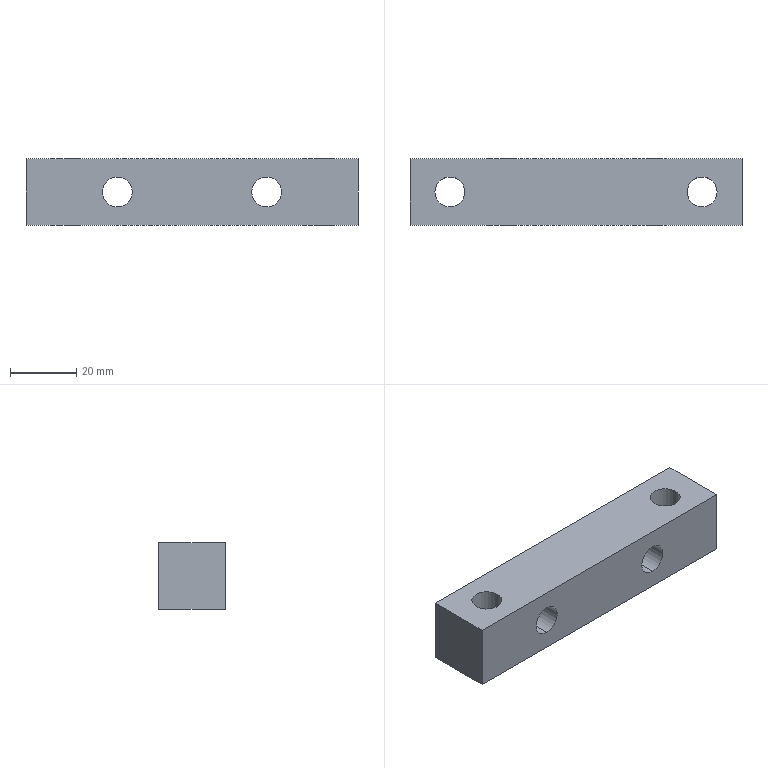Part | STEP file | 0244_218_Block | 1 solid | 14 faces | box 100 x 20 x 20 mm | volume 34911 mm3 | cylinder 8 | plane 6 | commonest cylinder face diameters 9 x8
STEP:
#1=CARTESIAN_POINT('',(0.,0.,0.));
#2=DIRECTION('',(0.,0.,1.));
#3=DIRECTION('',(1.,0.,0.));
#4=AXIS2_PLACEMENT_3D('',#1,#2,#3);
#5=CARTESIAN_POINT('',(-22.5,0.,5.5));
#6=VERTEX_POINT('',#5);
#7=CARTESIAN_POINT('',(-22.5,-20.,5.5));
#8=VERTEX_POINT('',#7);
#9=CARTESIAN_POINT('',(-22.5,-20.,5.5));
#10=DIRECTION('',(0.,-1.,0.));
#11=VECTOR('',#10,1.);
#12=LINE('',#9,#11);
#13=CARTESIAN_POINT('',(-22.5,-20.,10.));
#14=DIRECTION('',(0.,-1.,0.));
#15=DIRECTION('',(0.,0.,-1.));
#16=AXIS2_PLACEMENT_3D('',#13,#14,#15);
#17=CYLINDRICAL_SURFACE('',#16,4.5);
#18=CARTESIAN_POINT('',(6.283,0.));
#19=DIRECTION('',(0.,1.));
#20=VECTOR('',#19,1.);
#21=LINE('',#18,#20);
#22=(GEOMETRIC_REPRESENTATION_CONTEXT(2)PARAMETRIC_REPRESENTATION_CONTEXT()REPRESENTATION_CONTEXT('',''));
#23=DEFINITIONAL_REPRESENTATION('',(#21),#22);
#24=PCURVE('',#17,#23);
#25=CARTESIAN_POINT('',(-22.5,-20.,10.));
#26=DIRECTION('',(0.,-1.,0.));
#27=DIRECTION('',(0.,0.,-1.));
#28=AXIS2_PLACEMENT_3D('',#25,#26,#27);
#29=CYLINDRICAL_SURFACE('',#28,4.5);
#30=CARTESIAN_POINT('',(0.,0.));
#31=DIRECTION('',(0.,1.));
#32=VECTOR('',#31,1.);
#33=LINE('',#30,#32);
#34=(GEOMETRIC_REPRESENTATION_CONTEXT(2)PARAMETRIC_REPRESENTATION_CONTEXT()REPRESENTATION_CONTEXT('',''));
#35=DEFINITIONAL_REPRESENTATION('',(#33),#34);
#36=PCURVE('',#29,#35);
#37=SURFACE_CURVE('',#12,(#24,#36),.PCURVE_S1.);
#38=EDGE_CURVE('',#6,#8,#37,.T.);
#39=ORIENTED_EDGE('',*,*,#38,.T.);
#40=CARTESIAN_POINT('',(-22.5,-20.,14.5));
#41=VERTEX_POINT('',#40);
#42=CARTESIAN_POINT('',(-22.5,-20.,10.));
#43=DIRECTION('',(0.,-1.,0.));
#44=DIRECTION('',(0.,0.,-1.));
#45=AXIS2_PLACEMENT_3D('',#42,#43,#44);
#46=CIRCLE('',#45,4.5);
#47=CARTESIAN_POINT('',(0.,0.));
#48=DIRECTION('',(1.,0.));
#49=VECTOR('',#48,1.);
#50=LINE('',#47,#49);
#51=(GEOMETRIC_REPRESENTATION_CONTEXT(2)PARAMETRIC_REPRESENTATION_CONTEXT()REPRESENTATION_CONTEXT('',''));
#52=DEFINITIONAL_REPRESENTATION('',(#50),#51);
#53=PCURVE('',#17,#52);
#54=CARTESIAN_POINT('',(-50.,-20.,20.));
#55=DIRECTION('',(0.,1.,0.));
#56=DIRECTION('',(-1.,0.,0.));
#57=AXIS2_PLACEMENT_3D('',#54,#55,#56);
#58=PLANE('',#57);
#59=CARTESIAN_POINT('',(-27.5,-14.5));
#60=CARTESIAN_POINT('',(-35.294,-14.5));
#61=CARTESIAN_POINT('',(-31.397,-7.75));
#62=CARTESIAN_POINT('',(-27.5,-1.));
#63=CARTESIAN_POINT('',(-23.603,-7.75));
#64=CARTESIAN_POINT('',(-19.706,-14.5));
#65=CARTESIAN_POINT('',(-27.5,-14.5));
#66=(BOUNDED_CURVE()B_SPLINE_CURVE(2,(#59,#60,#61,#62,#63,#64,#65),.UNSPECIFIED.,.T.,.F.)B_SPLINE_CURVE_WITH_KNOTS((1,2,2,2,2,1),(-2.094,0.,2.094,4.189,6.283,8.378),.UNSPECIFIED.)CURVE()GEOMETRIC_REPRESENTATION_ITEM()RATIONAL_B_SPLINE_CURVE((1.,0.5,1.,0.5,1.,0.5,1.))REPRESENTATION_ITEM(''));
#67=(GEOMETRIC_REPRESENTATION_CONTEXT(2)PARAMETRIC_REPRESENTATION_CONTEXT()REPRESENTATION_CONTEXT('',''));
#68=DEFINITIONAL_REPRESENTATION('',(#66),#67);
#69=PCURVE('',#58,#68);
#70=SURFACE_CURVE('',#46,(#53,#69),.PCURVE_S1.);
#71=EDGE_CURVE('',#41,#8,#70,.T.);
#72=ORIENTED_EDGE('',*,*,#71,.F.);
#73=CARTESIAN_POINT('',(-22.5,0.,14.5));
#74=VERTEX_POINT('',#73);
#75=CARTESIAN_POINT('',(-22.5,-20.,14.5));
#76=DIRECTION('',(0.,-1.,0.));
#77=VECTOR('',#76,1.);
#78=LINE('',#75,#77);
#79=CARTESIAN_POINT('',(3.142,0.));
#80=DIRECTION('',(0.,1.));
#81=VECTOR('',#80,1.);
#82=LINE('',#79,#81);
#83=(GEOMETRIC_REPRESENTATION_CONTEXT(2)PARAMETRIC_REPRESENTATION_CONTEXT()REPRESENTATION_CONTEXT('',''));
#84=DEFINITIONAL_REPRESENTATION('',(#82),#83);
#85=PCURVE('',#17,#84);
#86=CARTESIAN_POINT('',(3.142,0.));
#87=DIRECTION('',(0.,1.));
#88=VECTOR('',#87,1.);
#89=LINE('',#86,#88);
#90=(GEOMETRIC_REPRESENTATION_CONTEXT(2)PARAMETRIC_REPRESENTATION_CONTEXT()REPRESENTATION_CONTEXT('',''));
#91=DEFINITIONAL_REPRESENTATION('',(#89),#90);
#92=PCURVE('',#29,#91);
#93=SURFACE_CURVE('',#78,(#85,#92),.PCURVE_S1.);
#94=EDGE_CURVE('',#74,#41,#93,.T.);
#95=ORIENTED_EDGE('',*,*,#94,.F.);
#96=CARTESIAN_POINT('',(-22.5,0.,10.));
#97=DIRECTION('',(0.,-1.,0.));
#98=DIRECTION('',(0.,0.,-1.));
#99=AXIS2_PLACEMENT_3D('',#96,#97,#98);
#100=CIRCLE('',#99,4.5);
#101=CARTESIAN_POINT('',(0.,-20.));
#102=DIRECTION('',(1.,0.));
#103=VECTOR('',#102,1.);
#104=LINE('',#101,#103);
#105=(GEOMETRIC_REPRESENTATION_CONTEXT(2)PARAMETRIC_REPRESENTATION_CONTEXT()REPRESENTATION_CONTEXT('',''));
#106=DEFINITIONAL_REPRESENTATION('',(#104),#105);
#107=PCURVE('',#17,#106);
#108=CARTESIAN_POINT('',(-50.,0.,20.));
#109=DIRECTION('',(0.,-1.,0.));
#110=DIRECTION('',(1.,0.,0.));
#111=AXIS2_PLACEMENT_3D('',#108,#109,#110);
#112=PLANE('',#111);
#113=CARTESIAN_POINT('',(27.5,-10.));
#114=DIRECTION('',(0.,-1.));
#115=AXIS2_PLACEMENT_2D('',#113,#114);
#116=CIRCLE('',#115,4.5);
#117=(GEOMETRIC_REPRESENTATION_CONTEXT(2)PARAMETRIC_REPRESENTATION_CONTEXT()REPRESENTATION_CONTEXT('',''));
#118=DEFINITIONAL_REPRESENTATION('',(#116),#117);
#119=PCURVE('',#112,#118);
#120=SURFACE_CURVE('',#100,(#107,#119),.PCURVE_S1.);
#121=EDGE_CURVE('',#74,#6,#120,.T.);
#122=ORIENTED_EDGE('',*,*,#121,.T.);
#123=EDGE_LOOP('',(#39,#72,#95,#122));
#124=FACE_BOUND('',#123,.F.);
#125=ADVANCED_FACE('',(#124),#17,.F.);
#126=CARTESIAN_POINT('',(22.5,0.,5.5));
#127=VERTEX_POINT('',#126);
#128=CARTESIAN_POINT('',(22.5,-20.,5.5));
#129=VERTEX_POINT('',#128);
#130=CARTESIAN_POINT('',(22.5,-20.,5.5));
#131=DIRECTION('',(0.,-1.,0.));
#132=VECTOR('',#131,1.);
#133=LINE('',#130,#132);
#134=CARTESIAN_POINT('',(22.5,-20.,10.));
#135=DIRECTION('',(0.,-1.,0.));
#136=DIRECTION('',(0.,0.,-1.));
#137=AXIS2_PLACEMENT_3D('',#134,#135,#136);
#138=CYLINDRICAL_SURFACE('',#137,4.5);
#139=CARTESIAN_POINT('',(6.283,0.));
#140=DIRECTION('',(0.,1.));
#141=VECTOR('',#140,1.);
#142=LINE('',#139,#141);
#143=(GEOMETRIC_REPRESENTATION_CONTEXT(2)PARAMETRIC_REPRESENTATION_CONTEXT()REPRESENTATION_CONTEXT('',''));
#144=DEFINITIONAL_REPRESENTATION('',(#142),#143);
#145=PCURVE('',#138,#144);
#146=CARTESIAN_POINT('',(22.5,-20.,10.));
#147=DIRECTION('',(0.,-1.,0.));
#148=DIRECTION('',(0.,0.,-1.));
#149=AXIS2_PLACEMENT_3D('',#146,#147,#148);
#150=CYLINDRICAL_SURFACE('',#149,4.5);
#151=CARTESIAN_POINT('',(0.,0.));
#152=DIRECTION('',(0.,1.));
#153=VECTOR('',#152,1.);
#154=LINE('',#151,#153);
#155=(GEOMETRIC_REPRESENTATION_CONTEXT(2)PARAMETRIC_REPRESENTATION_CONTEXT()REPRESENTATION_CONTEXT('',''));
#156=DEFINITIONAL_REPRESENTATION('',(#154),#155);
#157=PCURVE('',#150,#156);
#158=SURFACE_CURVE('',#133,(#145,#157),.PCURVE_S1.);
#159=EDGE_CURVE('',#127,#129,#158,.T.);
#160=ORIENTED_EDGE('',*,*,#159,.T.);
#161=CARTESIAN_POINT('',(22.5,-20.,14.5));
#162=VERTEX_POINT('',#161);
#163=CARTESIAN_POINT('',(22.5,-20.,10.));
#164=DIRECTION('',(0.,-1.,0.));
#165=DIRECTION('',(0.,0.,-1.));
#166=AXIS2_PLACEMENT_3D('',#163,#164,#165);
#167=CIRCLE('',#166,4.5);
#168=CARTESIAN_POINT('',(0.,0.));
#169=DIRECTION('',(1.,0.));
#170=VECTOR('',#169,1.);
#171=LINE('',#168,#170);
#172=(GEOMETRIC_REPRESENTATION_CONTEXT(2)PARAMETRIC_REPRESENTATION_CONTEXT()REPRESENTATION_CONTEXT('',''));
#173=DEFINITIONAL_REPRESENTATION('',(#171),#172);
#174=PCURVE('',#138,#173);
#175=CARTESIAN_POINT('',(-72.5,-14.5));
#176=CARTESIAN_POINT('',(-80.294,-14.5));
#177=CARTESIAN_POINT('',(-76.397,-7.75));
#178=CARTESIAN_POINT('',(-72.5,-1.));
#179=CARTESIAN_POINT('',(-68.603,-7.75));
#180=CARTESIAN_POINT('',(-64.706,-14.5));
#181=CARTESIAN_POINT('',(-72.5,-14.5));
#182=(BOUNDED_CURVE()B_SPLINE_CURVE(2,(#175,#176,#177,#178,#179,#180,#181),.UNSPECIFIED.,.T.,.F.)B_SPLINE_CURVE_WITH_KNOTS((1,2,2,2,2,1),(-2.094,0.,2.094,4.189,6.283,8.378),.UNSPECIFIED.)CURVE()GEOMETRIC_REPRESENTATION_ITEM()RATIONAL_B_SPLINE_CURVE((1.,0.5,1.,0.5,1.,0.5,1.))REPRESENTATION_ITEM(''));
#183=(GEOMETRIC_REPRESENTATION_CONTEXT(2)PARAMETRIC_REPRESENTATION_CONTEXT()REPRESENTATION_CONTEXT('',''));
#184=DEFINITIONAL_REPRESENTATION('',(#182),#183);
#185=PCURVE('',#58,#184);
#186=SURFACE_CURVE('',#167,(#174,#185),.PCURVE_S1.);
#187=EDGE_CURVE('',#162,#129,#186,.T.);
#188=ORIENTED_EDGE('',*,*,#187,.F.);
#189=CARTESIAN_POINT('',(22.5,0.,14.5));
#190=VERTEX_POINT('',#189);
#191=CARTESIAN_POINT('',(22.5,-20.,14.5));
#192=DIRECTION('',(0.,-1.,0.));
#193=VECTOR('',#192,1.);
#194=LINE('',#191,#193);
#195=CARTESIAN_POINT('',(3.142,0.));
#196=DIRECTION('',(0.,1.));
#197=VECTOR('',#196,1.);
#198=LINE('',#195,#197);
#199=(GEOMETRIC_REPRESENTATION_CONTEXT(2)PARAMETRIC_REPRESENTATION_CONTEXT()REPRESENTATION_CONTEXT('',''));
#200=DEFINITIONAL_REPRESENTATION('',(#198),#199);
#201=PCURVE('',#138,#200);
#202=CARTESIAN_POINT('',(3.142,0.));
#203=DIRECTION('',(0.,1.));
#204=VECTOR('',#203,1.);
#205=LINE('',#202,#204);
#206=(GEOMETRIC_REPRESENTATION_CONTEXT(2)PARAMETRIC_REPRESENTATION_CONTEXT()REPRESENTATION_CONTEXT('',''));
#207=DEFINITIONAL_REPRESENTATION('',(#205),#206);
#208=PCURVE('',#150,#207);
#209=SURFACE_CURVE('',#194,(#201,#208),.PCURVE_S1.);
#210=EDGE_CURVE('',#190,#162,#209,.T.);
#211=ORIENTED_EDGE('',*,*,#210,.F.);
#212=CARTESIAN_POINT('',(22.5,0.,10.));
#213=DIRECTION('',(0.,-1.,0.));
#214=DIRECTION('',(0.,0.,-1.));
#215=AXIS2_PLACEMENT_3D('',#212,#213,#214);
#216=CIRCLE('',#215,4.5);
#217=CARTESIAN_POINT('',(0.,-20.));
#218=DIRECTION('',(1.,0.));
#219=VECTOR('',#218,1.);
#220=LINE('',#217,#219);
#221=(GEOMETRIC_REPRESENTATION_CONTEXT(2)PARAMETRIC_REPRESENTATION_CONTEXT()REPRESENTATION_CONTEXT('',''));
#222=DEFINITIONAL_REPRESENTATION('',(#220),#221);
#223=PCURVE('',#138,#222);
#224=CARTESIAN_POINT('',(72.5,-10.));
#225=DIRECTION('',(0.,-1.));
#226=AXIS2_PLACEMENT_2D('',#224,#225);
#227=CIRCLE('',#226,4.5);
#228=(GEOMETRIC_REPRESENTATION_CONTEXT(2)PARAMETRIC_REPRESENTATION_CONTEXT()REPRESENTATION_CONTEXT('',''));
#229=DEFINITIONAL_REPRESENTATION('',(#227),#228);
#230=PCURVE('',#112,#229);
#231=SURFACE_CURVE('',#216,(#223,#230),.PCURVE_S1.);
#232=EDGE_CURVE('',#190,#127,#231,.T.);
#233=ORIENTED_EDGE('',*,*,#232,.T.);
#234=EDGE_LOOP('',(#160,#188,#211,#233));
#235=FACE_BOUND('',#234,.F.);
#236=ADVANCED_FACE('',(#235),#138,.F.);
#237=CARTESIAN_POINT('',(-33.5,-10.,0.));
#238=VERTEX_POINT('',#237);
#239=CARTESIAN_POINT('',(-33.5,-10.,20.));
#240=VERTEX_POINT('',#239);
#241=CARTESIAN_POINT('',(-33.5,-10.,20.));
#242=DIRECTION('',(0.,0.,1.));
#243=VECTOR('',#242,1.);
#244=LINE('',#241,#243);
#245=CARTESIAN_POINT('',(-38.,-10.,20.));
#246=DIRECTION('',(0.,0.,1.));
#247=DIRECTION('',(1.,0.,0.));
#248=AXIS2_PLACEMENT_3D('',#245,#246,#247);
#249=CYLINDRICAL_SURFACE('',#248,4.5);
#250=CARTESIAN_POINT('',(6.283,0.));
#251=DIRECTION('',(0.,1.));
#252=VECTOR('',#251,1.);
#253=LINE('',#250,#252);
#254=(GEOMETRIC_REPRESENTATION_CONTEXT(2)PARAMETRIC_REPRESENTATION_CONTEXT()REPRESENTATION_CONTEXT('',''));
#255=DEFINITIONAL_REPRESENTATION('',(#253),#254);
#256=PCURVE('',#249,#255);
#257=CARTESIAN_POINT('',(-38.,-10.,20.));
#258=DIRECTION('',(0.,0.,1.));
#259=DIRECTION('',(1.,0.,0.));
#260=AXIS2_PLACEMENT_3D('',#257,#258,#259);
#261=CYLINDRICAL_SURFACE('',#260,4.5);
#262=CARTESIAN_POINT('',(0.,0.));
#263=DIRECTION('',(0.,1.));
#264=VECTOR('',#263,1.);
#265=LINE('',#262,#264);
#266=(GEOMETRIC_REPRESENTATION_CONTEXT(2)PARAMETRIC_REPRESENTATION_CONTEXT()REPRESENTATION_CONTEXT('',''));
#267=DEFINITIONAL_REPRESENTATION('',(#265),#266);
#268=PCURVE('',#261,#267);
#269=SURFACE_CURVE('',#244,(#256,#268),.PCURVE_S1.);
#270=EDGE_CURVE('',#238,#240,#269,.T.);
#271=ORIENTED_EDGE('',*,*,#270,.T.);
#272=CARTESIAN_POINT('',(-42.5,-10.,20.));
#273=VERTEX_POINT('',#272);
#274=CARTESIAN_POINT('',(-38.,-10.,20.));
#275=DIRECTION('',(0.,0.,1.));
#276=DIRECTION('',(1.,0.,0.));
#277=AXIS2_PLACEMENT_3D('',#274,#275,#276);
#278=CIRCLE('',#277,4.5);
#279=CARTESIAN_POINT('',(0.,0.));
#280=DIRECTION('',(1.,0.));
#281=VECTOR('',#280,1.);
#282=LINE('',#279,#281);
#283=(GEOMETRIC_REPRESENTATION_CONTEXT(2)PARAMETRIC_REPRESENTATION_CONTEXT()REPRESENTATION_CONTEXT('',''));
#284=DEFINITIONAL_REPRESENTATION('',(#282),#283);
#285=PCURVE('',#249,#284);
#286=CARTESIAN_POINT('',(-50.,-20.,20.));
#287=DIRECTION('',(0.,0.,1.));
#288=DIRECTION('',(1.,0.,0.));
#289=AXIS2_PLACEMENT_3D('',#286,#287,#288);
#290=PLANE('',#289);
#291=CARTESIAN_POINT('',(12.,10.));
#292=DIRECTION('',(1.,0.));
#293=AXIS2_PLACEMENT_2D('',#291,#292);
#294=CIRCLE('',#293,4.5);
#295=(GEOMETRIC_REPRESENTATION_CONTEXT(2)PARAMETRIC_REPRESENTATION_CONTEXT()REPRESENTATION_CONTEXT('',''));
#296=DEFINITIONAL_REPRESENTATION('',(#294),#295);
#297=PCURVE('',#290,#296);
#298=SURFACE_CURVE('',#278,(#285,#297),.PCURVE_S1.);
#299=EDGE_CURVE('',#273,#240,#298,.T.);
#300=ORIENTED_EDGE('',*,*,#299,.F.);
#301=CARTESIAN_POINT('',(-42.5,-10.,0.));
#302=VERTEX_POINT('',#301);
#303=CARTESIAN_POINT('',(-42.5,-10.,20.));
#304=DIRECTION('',(0.,0.,1.));
#305=VECTOR('',#304,1.);
#306=LINE('',#303,#305);
#307=CARTESIAN_POINT('',(3.142,0.));
#308=DIRECTION('',(0.,1.));
#309=VECTOR('',#308,1.);
#310=LINE('',#307,#309);
#311=(GEOMETRIC_REPRESENTATION_CONTEXT(2)PARAMETRIC_REPRESENTATION_CONTEXT()REPRESENTATION_CONTEXT('',''));
#312=DEFINITIONAL_REPRESENTATION('',(#310),#311);
#313=PCURVE('',#249,#312);
#314=CARTESIAN_POINT('',(3.142,0.));
#315=DIRECTION('',(0.,1.));
#316=VECTOR('',#315,1.);
#317=LINE('',#314,#316);
#318=(GEOMETRIC_REPRESENTATION_CONTEXT(2)PARAMETRIC_REPRESENTATION_CONTEXT()REPRESENTATION_CONTEXT('',''));
#319=DEFINITIONAL_REPRESENTATION('',(#317),#318);
#320=PCURVE('',#261,#319);
#321=SURFACE_CURVE('',#306,(#313,#320),.PCURVE_S1.);
#322=EDGE_CURVE('',#302,#273,#321,.T.);
#323=ORIENTED_EDGE('',*,*,#322,.F.);
#324=CARTESIAN_POINT('',(-38.,-10.,0.));
#325=DIRECTION('',(0.,0.,1.));
#326=DIRECTION('',(1.,0.,0.));
#327=AXIS2_PLACEMENT_3D('',#324,#325,#326);
#328=CIRCLE('',#327,4.5);
#329=CARTESIAN_POINT('',(0.,-20.));
#330=DIRECTION('',(1.,0.));
#331=VECTOR('',#330,1.);
#332=LINE('',#329,#331);
#333=(GEOMETRIC_REPRESENTATION_CONTEXT(2)PARAMETRIC_REPRESENTATION_CONTEXT()REPRESENTATION_CONTEXT('',''));
#334=DEFINITIONAL_REPRESENTATION('',(#332),#333);
#335=PCURVE('',#249,#334);
#336=CARTESIAN_POINT('',(-50.,-20.,0.));
#337=DIRECTION('',(0.,0.,1.));
#338=DIRECTION('',(1.,0.,0.));
#339=AXIS2_PLACEMENT_3D('',#336,#337,#338);
#340=PLANE('',#339);
#341=CARTESIAN_POINT('',(12.,10.));
#342=DIRECTION('',(1.,0.));
#343=AXIS2_PLACEMENT_2D('',#341,#342);
#344=CIRCLE('',#343,4.5);
#345=(GEOMETRIC_REPRESENTATION_CONTEXT(2)PARAMETRIC_REPRESENTATION_CONTEXT()REPRESENTATION_CONTEXT('',''));
#346=DEFINITIONAL_REPRESENTATION('',(#344),#345);
#347=PCURVE('',#340,#346);
#348=SURFACE_CURVE('',#328,(#335,#347),.PCURVE_S1.);
#349=EDGE_CURVE('',#302,#238,#348,.T.);
#350=ORIENTED_EDGE('',*,*,#349,.T.);
#351=EDGE_LOOP('',(#271,#300,#323,#350));
#352=FACE_BOUND('',#351,.F.);
#353=ADVANCED_FACE('',(#352),#249,.F.);
#354=CARTESIAN_POINT('',(42.5,-10.,0.));
#355=VERTEX_POINT('',#354);
#356=CARTESIAN_POINT('',(42.5,-10.,20.));
#357=VERTEX_POINT('',#356);
#358=CARTESIAN_POINT('',(42.5,-10.,20.));
#359=DIRECTION('',(0.,0.,1.));
#360=VECTOR('',#359,1.);
#361=LINE('',#358,#360);
#362=CARTESIAN_POINT('',(38.,-10.,20.));
#363=DIRECTION('',(0.,0.,1.));
#364=DIRECTION('',(1.,0.,0.));
#365=AXIS2_PLACEMENT_3D('',#362,#363,#364);
#366=CYLINDRICAL_SURFACE('',#365,4.5);
#367=CARTESIAN_POINT('',(6.283,0.));
#368=DIRECTION('',(0.,1.));
#369=VECTOR('',#368,1.);
#370=LINE('',#367,#369);
#371=(GEOMETRIC_REPRESENTATION_CONTEXT(2)PARAMETRIC_REPRESENTATION_CONTEXT()REPRESENTATION_CONTEXT('',''));
#372=DEFINITIONAL_REPRESENTATION('',(#370),#371);
#373=PCURVE('',#366,#372);
#374=CARTESIAN_POINT('',(38.,-10.,20.));
#375=DIRECTION('',(0.,0.,1.));
#376=DIRECTION('',(1.,0.,0.));
#377=AXIS2_PLACEMENT_3D('',#374,#375,#376);
#378=CYLINDRICAL_SURFACE('',#377,4.5);
#379=CARTESIAN_POINT('',(0.,0.));
#380=DIRECTION('',(0.,1.));
#381=VECTOR('',#380,1.);
#382=LINE('',#379,#381);
#383=(GEOMETRIC_REPRESENTATION_CONTEXT(2)PARAMETRIC_REPRESENTATION_CONTEXT()REPRESENTATION_CONTEXT('',''));
#384=DEFINITIONAL_REPRESENTATION('',(#382),#383);
#385=PCURVE('',#378,#384);
#386=SURFACE_CURVE('',#361,(#373,#385),.PCURVE_S1.);
#387=EDGE_CURVE('',#355,#357,#386,.T.);
#388=ORIENTED_EDGE('',*,*,#387,.T.);
#389=CARTESIAN_POINT('',(33.5,-10.,20.));
#390=VERTEX_POINT('',#389);
#391=CARTESIAN_POINT('',(38.,-10.,20.));
#392=DIRECTION('',(0.,0.,1.));
#393=DIRECTION('',(1.,0.,0.));
#394=AXIS2_PLACEMENT_3D('',#391,#392,#393);
#395=CIRCLE('',#394,4.5);
#396=CARTESIAN_POINT('',(0.,0.));
#397=DIRECTION('',(1.,0.));
#398=VECTOR('',#397,1.);
#399=LINE('',#396,#398);
#400=(GEOMETRIC_REPRESENTATION_CONTEXT(2)PARAMETRIC_REPRESENTATION_CONTEXT()REPRESENTATION_CONTEXT('',''));
#401=DEFINITIONAL_REPRESENTATION('',(#399),#400);
#402=PCURVE('',#366,#401);
#403=CARTESIAN_POINT('',(88.,10.));
#404=DIRECTION('',(1.,0.));
#405=AXIS2_PLACEMENT_2D('',#403,#404);
#406=CIRCLE('',#405,4.5);
#407=(GEOMETRIC_REPRESENTATION_CONTEXT(2)PARAMETRIC_REPRESENTATION_CONTEXT()REPRESENTATION_CONTEXT('',''));
#408=DEFINITIONAL_REPRESENTATION('',(#406),#407);
#409=PCURVE('',#290,#408);
#410=SURFACE_CURVE('',#395,(#402,#409),.PCURVE_S1.);
#411=EDGE_CURVE('',#390,#357,#410,.T.);
#412=ORIENTED_EDGE('',*,*,#411,.F.);
#413=CARTESIAN_POINT('',(33.5,-10.,0.));
#414=VERTEX_POINT('',#413);
#415=CARTESIAN_POINT('',(33.5,-10.,20.));
#416=DIRECTION('',(0.,0.,1.));
#417=VECTOR('',#416,1.);
#418=LINE('',#415,#417);
#419=CARTESIAN_POINT('',(3.142,0.));
#420=DIRECTION('',(0.,1.));
#421=VECTOR('',#420,1.);
#422=LINE('',#419,#421);
#423=(GEOMETRIC_REPRESENTATION_CONTEXT(2)PARAMETRIC_REPRESENTATION_CONTEXT()REPRESENTATION_CONTEXT('',''));
#424=DEFINITIONAL_REPRESENTATION('',(#422),#423);
#425=PCURVE('',#366,#424);
#426=CARTESIAN_POINT('',(3.142,0.));
#427=DIRECTION('',(0.,1.));
#428=VECTOR('',#427,1.);
#429=LINE('',#426,#428);
#430=(GEOMETRIC_REPRESENTATION_CONTEXT(2)PARAMETRIC_REPRESENTATION_CONTEXT()REPRESENTATION_CONTEXT('',''));
#431=DEFINITIONAL_REPRESENTATION('',(#429),#430);
#432=PCURVE('',#378,#431);
#433=SURFACE_CURVE('',#418,(#425,#432),.PCURVE_S1.);
#434=EDGE_CURVE('',#414,#390,#433,.T.);
#435=ORIENTED_EDGE('',*,*,#434,.F.);
#436=CARTESIAN_POINT('',(38.,-10.,0.));
#437=DIRECTION('',(0.,0.,1.));
#438=DIRECTION('',(1.,0.,0.));
#439=AXIS2_PLACEMENT_3D('',#436,#437,#438);
#440=CIRCLE('',#439,4.5);
#441=CARTESIAN_POINT('',(0.,-20.));
#442=DIRECTION('',(1.,0.));
#443=VECTOR('',#442,1.);
#444=LINE('',#441,#443);
#445=(GEOMETRIC_REPRESENTATION_CONTEXT(2)PARAMETRIC_REPRESENTATION_CONTEXT()REPRESENTATION_CONTEXT('',''));
#446=DEFINITIONAL_REPRESENTATION('',(#444),#445);
#447=PCURVE('',#366,#446);
#448=CARTESIAN_POINT('',(88.,10.));
#449=DIRECTION('',(1.,0.));
#450=AXIS2_PLACEMENT_2D('',#448,#449);
#451=CIRCLE('',#450,4.5);
#452=(GEOMETRIC_REPRESENTATION_CONTEXT(2)PARAMETRIC_REPRESENTATION_CONTEXT()REPRESENTATION_CONTEXT('',''));
#453=DEFINITIONAL_REPRESENTATION('',(#451),#452);
#454=PCURVE('',#340,#453);
#455=SURFACE_CURVE('',#440,(#447,#454),.PCURVE_S1.);
#456=EDGE_CURVE('',#414,#355,#455,.T.);
#457=ORIENTED_EDGE('',*,*,#456,.T.);
#458=EDGE_LOOP('',(#388,#412,#435,#457));
#459=FACE_BOUND('',#458,.F.);
#460=ADVANCED_FACE('',(#459),#366,.F.);
#461=CARTESIAN_POINT('',(-50.,0.,0.));
#462=VERTEX_POINT('',#461);
#463=CARTESIAN_POINT('',(-50.,-20.,0.));
#464=VERTEX_POINT('',#463);
#465=CARTESIAN_POINT('',(-50.,0.,0.));
#466=DIRECTION('',(0.,-1.,0.));
#467=VECTOR('',#466,1.);
#468=LINE('',#465,#467);
#469=CARTESIAN_POINT('',(-50.,0.,20.));
#470=DIRECTION('',(1.,0.,0.));
#471=DIRECTION('',(0.,0.,-1.));
#472=AXIS2_PLACEMENT_3D('',#469,#470,#471);
#473=PLANE('',#472);
#474=CARTESIAN_POINT('',(20.,0.));
#475=DIRECTION('',(0.,-1.));
#476=VECTOR('',#475,1.);
#477=LINE('',#474,#476);
#478=(GEOMETRIC_REPRESENTATION_CONTEXT(2)PARAMETRIC_REPRESENTATION_CONTEXT()REPRESENTATION_CONTEXT('',''));
#479=DEFINITIONAL_REPRESENTATION('',(#477),#478);
#480=PCURVE('',#473,#479);
#481=CARTESIAN_POINT('',(0.,20.));
#482=DIRECTION('',(0.,-1.));
#483=VECTOR('',#482,1.);
#484=LINE('',#481,#483);
#485=(GEOMETRIC_REPRESENTATION_CONTEXT(2)PARAMETRIC_REPRESENTATION_CONTEXT()REPRESENTATION_CONTEXT('',''));
#486=DEFINITIONAL_REPRESENTATION('',(#484),#485);
#487=PCURVE('',#340,#486);
#488=SURFACE_CURVE('',#468,(#480,#487),.PCURVE_S1.);
#489=EDGE_CURVE('',#462,#464,#488,.T.);
#490=ORIENTED_EDGE('',*,*,#489,.T.);
#491=CARTESIAN_POINT('',(-50.,-20.,20.));
#492=VERTEX_POINT('',#491);
#493=CARTESIAN_POINT('',(-50.,-20.,20.));
#494=DIRECTION('',(0.,0.,-1.));
#495=VECTOR('',#494,1.);
#496=LINE('',#493,#495);
#497=CARTESIAN_POINT('',(0.,-20.));
#498=DIRECTION('',(1.,0.));
#499=VECTOR('',#498,1.);
#500=LINE('',#497,#499);
#501=(GEOMETRIC_REPRESENTATION_CONTEXT(2)PARAMETRIC_REPRESENTATION_CONTEXT()REPRESENTATION_CONTEXT('',''));
#502=DEFINITIONAL_REPRESENTATION('',(#500),#501);
#503=PCURVE('',#473,#502);
#504=CARTESIAN_POINT('',(0.,0.));
#505=DIRECTION('',(0.,-1.));
#506=VECTOR('',#505,1.);
#507=LINE('',#504,#506);
#508=(GEOMETRIC_REPRESENTATION_CONTEXT(2)PARAMETRIC_REPRESENTATION_CONTEXT()REPRESENTATION_CONTEXT('',''));
#509=DEFINITIONAL_REPRESENTATION('',(#507),#508);
#510=PCURVE('',#58,#509);
#511=SURFACE_CURVE('',#496,(#503,#510),.PCURVE_S1.);
#512=EDGE_CURVE('',#492,#464,#511,.T.);
#513=ORIENTED_EDGE('',*,*,#512,.F.);
#514=CARTESIAN_POINT('',(-50.,0.,20.));
#515=VERTEX_POINT('',#514);
#516=CARTESIAN_POINT('',(-50.,0.,20.));
#517=DIRECTION('',(0.,-1.,0.));
#518=VECTOR('',#517,1.);
#519=LINE('',#516,#518);
#520=CARTESIAN_POINT('',(0.,0.));
#521=DIRECTION('',(0.,-1.));
#522=VECTOR('',#521,1.);
#523=LINE('',#520,#522);
#524=(GEOMETRIC_REPRESENTATION_CONTEXT(2)PARAMETRIC_REPRESENTATION_CONTEXT()REPRESENTATION_CONTEXT('',''));
#525=DEFINITIONAL_REPRESENTATION('',(#523),#524);
#526=PCURVE('',#473,#525);
#527=CARTESIAN_POINT('',(0.,20.));
#528=DIRECTION('',(0.,-1.));
#529=VECTOR('',#528,1.);
#530=LINE('',#527,#529);
#531=(GEOMETRIC_REPRESENTATION_CONTEXT(2)PARAMETRIC_REPRESENTATION_CONTEXT()REPRESENTATION_CONTEXT('',''));
#532=DEFINITIONAL_REPRESENTATION('',(#530),#531);
#533=PCURVE('',#290,#532);
#534=SURFACE_CURVE('',#519,(#526,#533),.PCURVE_S1.);
#535=EDGE_CURVE('',#515,#492,#534,.T.);
#536=ORIENTED_EDGE('',*,*,#535,.F.);
#537=CARTESIAN_POINT('',(-50.,0.,20.));
#538=DIRECTION('',(0.,0.,-1.));
#539=VECTOR('',#538,1.);
#540=LINE('',#537,#539);
#541=CARTESIAN_POINT('',(0.,0.));
#542=DIRECTION('',(1.,0.));
#543=VECTOR('',#542,1.);
#544=LINE('',#541,#543);
#545=(GEOMETRIC_REPRESENTATION_CONTEXT(2)PARAMETRIC_REPRESENTATION_CONTEXT()REPRESENTATION_CONTEXT('',''));
#546=DEFINITIONAL_REPRESENTATION('',(#544),#545);
#547=PCURVE('',#473,#546);
#548=CARTESIAN_POINT('',(0.,0.));
#549=DIRECTION('',(0.,-1.));
#550=VECTOR('',#549,1.);
#551=LINE('',#548,#550);
#552=(GEOMETRIC_REPRESENTATION_CONTEXT(2)PARAMETRIC_REPRESENTATION_CONTEXT()REPRESENTATION_CONTEXT('',''));
#553=DEFINITIONAL_REPRESENTATION('',(#551),#552);
#554=PCURVE('',#112,#553);
#555=SURFACE_CURVE('',#540,(#547,#554),.PCURVE_S1.);
#556=EDGE_CURVE('',#515,#462,#555,.T.);
#557=ORIENTED_EDGE('',*,*,#556,.T.);
#558=EDGE_LOOP('',(#490,#513,#536,#557));
#559=FACE_BOUND('',#558,.T.);
#560=ADVANCED_FACE('',(#559),#473,.F.);
#561=CARTESIAN_POINT('',(-22.5,-20.,10.));
#562=DIRECTION('',(0.,-1.,0.));
#563=DIRECTION('',(0.,0.,-1.));
#564=AXIS2_PLACEMENT_3D('',#561,#562,#563);
#565=CIRCLE('',#564,4.5);
#566=CARTESIAN_POINT('',(-27.5,-14.5));
#567=CARTESIAN_POINT('',(-35.294,-14.5));
#568=CARTESIAN_POINT('',(-31.397,-7.75));
#569=CARTESIAN_POINT('',(-27.5,-1.));
#570=CARTESIAN_POINT('',(-23.603,-7.75));
#571=CARTESIAN_POINT('',(-19.706,-14.5));
#572=CARTESIAN_POINT('',(-27.5,-14.5));
#573=(BOUNDED_CURVE()B_SPLINE_CURVE(2,(#566,#567,#568,#569,#570,#571,#572),.UNSPECIFIED.,.T.,.F.)B_SPLINE_CURVE_WITH_KNOTS((1,2,2,2,2,1),(-2.094,0.,2.094,4.189,6.283,8.378),.UNSPECIFIED.)CURVE()GEOMETRIC_REPRESENTATION_ITEM()RATIONAL_B_SPLINE_CURVE((1.,0.5,1.,0.5,1.,0.5,1.))REPRESENTATION_ITEM(''));
#574=(GEOMETRIC_REPRESENTATION_CONTEXT(2)PARAMETRIC_REPRESENTATION_CONTEXT()REPRESENTATION_CONTEXT('',''));
#575=DEFINITIONAL_REPRESENTATION('',(#573),#574);
#576=PCURVE('',#58,#575);
#577=CARTESIAN_POINT('',(0.,0.));
#578=DIRECTION('',(1.,0.));
#579=VECTOR('',#578,1.);
#580=LINE('',#577,#579);
#581=(GEOMETRIC_REPRESENTATION_CONTEXT(2)PARAMETRIC_REPRESENTATION_CONTEXT()REPRESENTATION_CONTEXT('',''));
#582=DEFINITIONAL_REPRESENTATION('',(#580),#581);
#583=PCURVE('',#29,#582);
#584=SURFACE_CURVE('',#565,(#576,#583),.PCURVE_S1.);
#585=EDGE_CURVE('',#8,#41,#584,.T.);
#586=ORIENTED_EDGE('',*,*,#585,.F.);
#587=ORIENTED_EDGE('',*,*,#71,.F.);
#588=EDGE_LOOP('',(#586,#587));
#589=FACE_BOUND('',#588,.T.);
#590=CARTESIAN_POINT('',(22.5,-20.,10.));
#591=DIRECTION('',(0.,-1.,0.));
#592=DIRECTION('',(0.,0.,-1.));
#593=AXIS2_PLACEMENT_3D('',#590,#591,#592);
#594=CIRCLE('',#593,4.5);
#595=CARTESIAN_POINT('',(-72.5,-14.5));
#596=CARTESIAN_POINT('',(-80.294,-14.5));
#597=CARTESIAN_POINT('',(-76.397,-7.75));
#598=CARTESIAN_POINT('',(-72.5,-1.));
#599=CARTESIAN_POINT('',(-68.603,-7.75));
#600=CARTESIAN_POINT('',(-64.706,-14.5));
#601=CARTESIAN_POINT('',(-72.5,-14.5));
#602=(BOUNDED_CURVE()B_SPLINE_CURVE(2,(#595,#596,#597,#598,#599,#600,#601),.UNSPECIFIED.,.T.,.F.)B_SPLINE_CURVE_WITH_KNOTS((1,2,2,2,2,1),(-2.094,0.,2.094,4.189,6.283,8.378),.UNSPECIFIED.)CURVE()GEOMETRIC_REPRESENTATION_ITEM()RATIONAL_B_SPLINE_CURVE((1.,0.5,1.,0.5,1.,0.5,1.))REPRESENTATION_ITEM(''));
#603=(GEOMETRIC_REPRESENTATION_CONTEXT(2)PARAMETRIC_REPRESENTATION_CONTEXT()REPRESENTATION_CONTEXT('',''));
#604=DEFINITIONAL_REPRESENTATION('',(#602),#603);
#605=PCURVE('',#58,#604);
#606=CARTESIAN_POINT('',(0.,0.));
#607=DIRECTION('',(1.,0.));
#608=VECTOR('',#607,1.);
#609=LINE('',#606,#608);
#610=(GEOMETRIC_REPRESENTATION_CONTEXT(2)PARAMETRIC_REPRESENTATION_CONTEXT()REPRESENTATION_CONTEXT('',''));
#611=DEFINITIONAL_REPRESENTATION('',(#609),#610);
#612=PCURVE('',#150,#611);
#613=SURFACE_CURVE('',#594,(#605,#612),.PCURVE_S1.);
#614=EDGE_CURVE('',#129,#162,#613,.T.);
#615=ORIENTED_EDGE('',*,*,#614,.F.);
#616=ORIENTED_EDGE('',*,*,#187,.F.);
#617=EDGE_LOOP('',(#615,#616));
#618=FACE_BOUND('',#617,.T.);
#619=CARTESIAN_POINT('',(50.,-20.,0.));
#620=VERTEX_POINT('',#619);
#621=CARTESIAN_POINT('',(-50.,-20.,0.));
#622=DIRECTION('',(1.,0.,0.));
#623=VECTOR('',#622,1.);
#624=LINE('',#621,#623);
#625=CARTESIAN_POINT('',(0.,-20.));
#626=DIRECTION('',(-1.,0.));
#627=VECTOR('',#626,1.);
#628=LINE('',#625,#627);
#629=(GEOMETRIC_REPRESENTATION_CONTEXT(2)PARAMETRIC_REPRESENTATION_CONTEXT()REPRESENTATION_CONTEXT('',''));
#630=DEFINITIONAL_REPRESENTATION('',(#628),#629);
#631=PCURVE('',#58,#630);
#632=CARTESIAN_POINT('',(0.,0.));
#633=DIRECTION('',(1.,0.));
#634=VECTOR('',#633,1.);
#635=LINE('',#632,#634);
#636=(GEOMETRIC_REPRESENTATION_CONTEXT(2)PARAMETRIC_REPRESENTATION_CONTEXT()REPRESENTATION_CONTEXT('',''));
#637=DEFINITIONAL_REPRESENTATION('',(#635),#636);
#638=PCURVE('',#340,#637);
#639=SURFACE_CURVE('',#624,(#631,#638),.PCURVE_S1.);
#640=EDGE_CURVE('',#464,#620,#639,.T.);
#641=ORIENTED_EDGE('',*,*,#640,.T.);
#642=CARTESIAN_POINT('',(50.,-20.,20.));
#643=VERTEX_POINT('',#642);
#644=CARTESIAN_POINT('',(50.,-20.,20.));
#645=DIRECTION('',(0.,0.,-1.));
#646=VECTOR('',#645,1.);
#647=LINE('',#644,#646);
#648=CARTESIAN_POINT('',(-100.,0.));
#649=DIRECTION('',(0.,-1.));
#650=VECTOR('',#649,1.);
#651=LINE('',#648,#650);
#652=(GEOMETRIC_REPRESENTATION_CONTEXT(2)PARAMETRIC_REPRESENTATION_CONTEXT()REPRESENTATION_CONTEXT('',''));
#653=DEFINITIONAL_REPRESENTATION('',(#651),#652);
#654=PCURVE('',#58,#653);
#655=CARTESIAN_POINT('',(50.,0.,20.));
#656=DIRECTION('',(-1.,0.,0.));
#657=DIRECTION('',(0.,0.,1.));
#658=AXIS2_PLACEMENT_3D('',#655,#656,#657);
#659=PLANE('',#658);
#660=CARTESIAN_POINT('',(0.,-20.));
#661=DIRECTION('',(-1.,0.));
#662=VECTOR('',#661,1.);
#663=LINE('',#660,#662);
#664=(GEOMETRIC_REPRESENTATION_CONTEXT(2)PARAMETRIC_REPRESENTATION_CONTEXT()REPRESENTATION_CONTEXT('',''));
#665=DEFINITIONAL_REPRESENTATION('',(#663),#664);
#666=PCURVE('',#659,#665);
#667=SURFACE_CURVE('',#647,(#654,#666),.PCURVE_S1.);
#668=EDGE_CURVE('',#643,#620,#667,.T.);
#669=ORIENTED_EDGE('',*,*,#668,.F.);
#670=CARTESIAN_POINT('',(-50.,-20.,20.));
#671=DIRECTION('',(1.,0.,0.));
#672=VECTOR('',#671,1.);
#673=LINE('',#670,#672);
#674=CARTESIAN_POINT('',(0.,0.));
#675=DIRECTION('',(-1.,0.));
#676=VECTOR('',#675,1.);
#677=LINE('',#674,#676);
#678=(GEOMETRIC_REPRESENTATION_CONTEXT(2)PARAMETRIC_REPRESENTATION_CONTEXT()REPRESENTATION_CONTEXT('',''));
#679=DEFINITIONAL_REPRESENTATION('',(#677),#678);
#680=PCURVE('',#58,#679);
#681=CARTESIAN_POINT('',(0.,0.));
#682=DIRECTION('',(1.,0.));
#683=VECTOR('',#682,1.);
#684=LINE('',#681,#683);
#685=(GEOMETRIC_REPRESENTATION_CONTEXT(2)PARAMETRIC_REPRESENTATION_CONTEXT()REPRESENTATION_CONTEXT('',''));
#686=DEFINITIONAL_REPRESENTATION('',(#684),#685);
#687=PCURVE('',#290,#686);
#688=SURFACE_CURVE('',#673,(#680,#687),.PCURVE_S1.);
#689=EDGE_CURVE('',#492,#643,#688,.T.);
#690=ORIENTED_EDGE('',*,*,#689,.F.);
#691=ORIENTED_EDGE('',*,*,#512,.T.);
#692=EDGE_LOOP('',(#641,#669,#690,#691));
#693=FACE_BOUND('',#692,.T.);
#694=ADVANCED_FACE('',(#589,#618,#693),#58,.F.);
#695=CARTESIAN_POINT('',(50.,0.,0.));
#696=VERTEX_POINT('',#695);
#697=CARTESIAN_POINT('',(50.,0.,0.));
#698=DIRECTION('',(0.,1.,0.));
#699=VECTOR('',#698,1.);
#700=LINE('',#697,#699);
#701=CARTESIAN_POINT('',(-20.,0.));
#702=DIRECTION('',(0.,1.));
#703=VECTOR('',#702,1.);
#704=LINE('',#701,#703);
#705=(GEOMETRIC_REPRESENTATION_CONTEXT(2)PARAMETRIC_REPRESENTATION_CONTEXT()REPRESENTATION_CONTEXT('',''));
#706=DEFINITIONAL_REPRESENTATION('',(#704),#705);
#707=PCURVE('',#659,#706);
#708=CARTESIAN_POINT('',(100.,20.));
#709=DIRECTION('',(0.,1.));
#710=VECTOR('',#709,1.);
#711=LINE('',#708,#710);
#712=(GEOMETRIC_REPRESENTATION_CONTEXT(2)PARAMETRIC_REPRESENTATION_CONTEXT()REPRESENTATION_CONTEXT('',''));
#713=DEFINITIONAL_REPRESENTATION('',(#711),#712);
#714=PCURVE('',#340,#713);
#715=SURFACE_CURVE('',#700,(#707,#714),.PCURVE_S1.);
#716=EDGE_CURVE('',#620,#696,#715,.T.);
#717=ORIENTED_EDGE('',*,*,#716,.T.);
#718=CARTESIAN_POINT('',(50.,0.,20.));
#719=VERTEX_POINT('',#718);
#720=CARTESIAN_POINT('',(50.,0.,20.));
#721=DIRECTION('',(0.,0.,-1.));
#722=VECTOR('',#721,1.);
#723=LINE('',#720,#722);
#724=CARTESIAN_POINT('',(0.,0.));
#725=DIRECTION('',(-1.,0.));
#726=VECTOR('',#725,1.);
#727=LINE('',#724,#726);
#728=(GEOMETRIC_REPRESENTATION_CONTEXT(2)PARAMETRIC_REPRESENTATION_CONTEXT()REPRESENTATION_CONTEXT('',''));
#729=DEFINITIONAL_REPRESENTATION('',(#727),#728);
#730=PCURVE('',#659,#729);
#731=CARTESIAN_POINT('',(100.,0.));
#732=DIRECTION('',(0.,-1.));
#733=VECTOR('',#732,1.);
#734=LINE('',#731,#733);
#735=(GEOMETRIC_REPRESENTATION_CONTEXT(2)PARAMETRIC_REPRESENTATION_CONTEXT()REPRESENTATION_CONTEXT('',''));
#736=DEFINITIONAL_REPRESENTATION('',(#734),#735);
#737=PCURVE('',#112,#736);
#738=SURFACE_CURVE('',#723,(#730,#737),.PCURVE_S1.);
#739=EDGE_CURVE('',#719,#696,#738,.T.);
#740=ORIENTED_EDGE('',*,*,#739,.F.);
#741=CARTESIAN_POINT('',(50.,0.,20.));
#742=DIRECTION('',(0.,1.,0.));
#743=VECTOR('',#742,1.);
#744=LINE('',#741,#743);
#745=CARTESIAN_POINT('',(0.,0.));
#746=DIRECTION('',(0.,1.));
#747=VECTOR('',#746,1.);
#748=LINE('',#745,#747);
#749=(GEOMETRIC_REPRESENTATION_CONTEXT(2)PARAMETRIC_REPRESENTATION_CONTEXT()REPRESENTATION_CONTEXT('',''));
#750=DEFINITIONAL_REPRESENTATION('',(#748),#749);
#751=PCURVE('',#659,#750);
#752=CARTESIAN_POINT('',(100.,20.));
#753=DIRECTION('',(0.,1.));
#754=VECTOR('',#753,1.);
#755=LINE('',#752,#754);
#756=(GEOMETRIC_REPRESENTATION_CONTEXT(2)PARAMETRIC_REPRESENTATION_CONTEXT()REPRESENTATION_CONTEXT('',''));
#757=DEFINITIONAL_REPRESENTATION('',(#755),#756);
#758=PCURVE('',#290,#757);
#759=SURFACE_CURVE('',#744,(#751,#758),.PCURVE_S1.);
#760=EDGE_CURVE('',#643,#719,#759,.T.);
#761=ORIENTED_EDGE('',*,*,#760,.F.);
#762=ORIENTED_EDGE('',*,*,#668,.T.);
#763=EDGE_LOOP('',(#717,#740,#761,#762));
#764=FACE_BOUND('',#763,.T.);
#765=ADVANCED_FACE('',(#764),#659,.F.);
#766=CARTESIAN_POINT('',(-22.5,0.,10.));
#767=DIRECTION('',(0.,-1.,0.));
#768=DIRECTION('',(0.,0.,-1.));
#769=AXIS2_PLACEMENT_3D('',#766,#767,#768);
#770=CIRCLE('',#769,4.5);
#771=CARTESIAN_POINT('',(27.5,-10.));
#772=DIRECTION('',(0.,-1.));
#773=AXIS2_PLACEMENT_2D('',#771,#772);
#774=CIRCLE('',#773,4.5);
#775=(GEOMETRIC_REPRESENTATION_CONTEXT(2)PARAMETRIC_REPRESENTATION_CONTEXT()REPRESENTATION_CONTEXT('',''));
#776=DEFINITIONAL_REPRESENTATION('',(#774),#775);
#777=PCURVE('',#112,#776);
#778=CARTESIAN_POINT('',(0.,-20.));
#779=DIRECTION('',(1.,0.));
#780=VECTOR('',#779,1.);
#781=LINE('',#778,#780);
#782=(GEOMETRIC_REPRESENTATION_CONTEXT(2)PARAMETRIC_REPRESENTATION_CONTEXT()REPRESENTATION_CONTEXT('',''));
#783=DEFINITIONAL_REPRESENTATION('',(#781),#782);
#784=PCURVE('',#29,#783);
#785=SURFACE_CURVE('',#770,(#777,#784),.PCURVE_S1.);
#786=EDGE_CURVE('',#6,#74,#785,.T.);
#787=ORIENTED_EDGE('',*,*,#786,.T.);
#788=ORIENTED_EDGE('',*,*,#121,.T.);
#789=EDGE_LOOP('',(#787,#788));
#790=FACE_BOUND('',#789,.T.);
#791=CARTESIAN_POINT('',(22.5,0.,10.));
#792=DIRECTION('',(0.,-1.,0.));
#793=DIRECTION('',(0.,0.,-1.));
#794=AXIS2_PLACEMENT_3D('',#791,#792,#793);
#795=CIRCLE('',#794,4.5);
#796=CARTESIAN_POINT('',(72.5,-10.));
#797=DIRECTION('',(0.,-1.));
#798=AXIS2_PLACEMENT_2D('',#796,#797);
#799=CIRCLE('',#798,4.5);
#800=(GEOMETRIC_REPRESENTATION_CONTEXT(2)PARAMETRIC_REPRESENTATION_CONTEXT()REPRESENTATION_CONTEXT('',''));
#801=DEFINITIONAL_REPRESENTATION('',(#799),#800);
#802=PCURVE('',#112,#801);
#803=CARTESIAN_POINT('',(0.,-20.));
#804=DIRECTION('',(1.,0.));
#805=VECTOR('',#804,1.);
#806=LINE('',#803,#805);
#807=(GEOMETRIC_REPRESENTATION_CONTEXT(2)PARAMETRIC_REPRESENTATION_CONTEXT()REPRESENTATION_CONTEXT('',''));
#808=DEFINITIONAL_REPRESENTATION('',(#806),#807);
#809=PCURVE('',#150,#808);
#810=SURFACE_CURVE('',#795,(#802,#809),.PCURVE_S1.);
#811=EDGE_CURVE('',#127,#190,#810,.T.);
#812=ORIENTED_EDGE('',*,*,#811,.T.);
#813=ORIENTED_EDGE('',*,*,#232,.T.);
#814=EDGE_LOOP('',(#812,#813));
#815=FACE_BOUND('',#814,.T.);
#816=CARTESIAN_POINT('',(-50.,0.,0.));
#817=DIRECTION('',(-1.,0.,0.));
#818=VECTOR('',#817,1.);
#819=LINE('',#816,#818);
#820=CARTESIAN_POINT('',(0.,-20.));
#821=DIRECTION('',(-1.,0.));
#822=VECTOR('',#821,1.);
#823=LINE('',#820,#822);
#824=(GEOMETRIC_REPRESENTATION_CONTEXT(2)PARAMETRIC_REPRESENTATION_CONTEXT()REPRESENTATION_CONTEXT('',''));
#825=DEFINITIONAL_REPRESENTATION('',(#823),#824);
#826=PCURVE('',#112,#825);
#827=CARTESIAN_POINT('',(0.,20.));
#828=DIRECTION('',(-1.,0.));
#829=VECTOR('',#828,1.);
#830=LINE('',#827,#829);
#831=(GEOMETRIC_REPRESENTATION_CONTEXT(2)PARAMETRIC_REPRESENTATION_CONTEXT()REPRESENTATION_CONTEXT('',''));
#832=DEFINITIONAL_REPRESENTATION('',(#830),#831);
#833=PCURVE('',#340,#832);
#834=SURFACE_CURVE('',#819,(#826,#833),.PCURVE_S1.);
#835=EDGE_CURVE('',#696,#462,#834,.T.);
#836=ORIENTED_EDGE('',*,*,#835,.T.);
#837=ORIENTED_EDGE('',*,*,#556,.F.);
#838=CARTESIAN_POINT('',(-50.,0.,20.));
#839=DIRECTION('',(-1.,0.,0.));
#840=VECTOR('',#839,1.);
#841=LINE('',#838,#840);
#842=CARTESIAN_POINT('',(0.,0.));
#843=DIRECTION('',(-1.,0.));
#844=VECTOR('',#843,1.);
#845=LINE('',#842,#844);
#846=(GEOMETRIC_REPRESENTATION_CONTEXT(2)PARAMETRIC_REPRESENTATION_CONTEXT()REPRESENTATION_CONTEXT('',''));
#847=DEFINITIONAL_REPRESENTATION('',(#845),#846);
#848=PCURVE('',#112,#847);
#849=CARTESIAN_POINT('',(0.,20.));
#850=DIRECTION('',(-1.,0.));
#851=VECTOR('',#850,1.);
#852=LINE('',#849,#851);
#853=(GEOMETRIC_REPRESENTATION_CONTEXT(2)PARAMETRIC_REPRESENTATION_CONTEXT()REPRESENTATION_CONTEXT('',''));
#854=DEFINITIONAL_REPRESENTATION('',(#852),#853);
#855=PCURVE('',#290,#854);
#856=SURFACE_CURVE('',#841,(#848,#855),.PCURVE_S1.);
#857=EDGE_CURVE('',#719,#515,#856,.T.);
#858=ORIENTED_EDGE('',*,*,#857,.F.);
#859=ORIENTED_EDGE('',*,*,#739,.T.);
#860=EDGE_LOOP('',(#836,#837,#858,#859));
#861=FACE_BOUND('',#860,.T.);
#862=ADVANCED_FACE('',(#790,#815,#861),#112,.F.);
#863=CARTESIAN_POINT('',(-38.,-10.,20.));
#864=DIRECTION('',(0.,0.,1.));
#865=DIRECTION('',(1.,0.,0.));
#866=AXIS2_PLACEMENT_3D('',#863,#864,#865);
#867=CIRCLE('',#866,4.5);
#868=CARTESIAN_POINT('',(12.,10.));
#869=DIRECTION('',(1.,0.));
#870=AXIS2_PLACEMENT_2D('',#868,#869);
#871=CIRCLE('',#870,4.5);
#872=(GEOMETRIC_REPRESENTATION_CONTEXT(2)PARAMETRIC_REPRESENTATION_CONTEXT()REPRESENTATION_CONTEXT('',''));
#873=DEFINITIONAL_REPRESENTATION('',(#871),#872);
#874=PCURVE('',#290,#873);
#875=CARTESIAN_POINT('',(0.,0.));
#876=DIRECTION('',(1.,0.));
#877=VECTOR('',#876,1.);
#878=LINE('',#875,#877);
#879=(GEOMETRIC_REPRESENTATION_CONTEXT(2)PARAMETRIC_REPRESENTATION_CONTEXT()REPRESENTATION_CONTEXT('',''));
#880=DEFINITIONAL_REPRESENTATION('',(#878),#879);
#881=PCURVE('',#261,#880);
#882=SURFACE_CURVE('',#867,(#874,#881),.PCURVE_S1.);
#883=EDGE_CURVE('',#240,#273,#882,.T.);
#884=ORIENTED_EDGE('',*,*,#883,.F.);
#885=ORIENTED_EDGE('',*,*,#299,.F.);
#886=EDGE_LOOP('',(#884,#885));
#887=FACE_BOUND('',#886,.T.);
#888=CARTESIAN_POINT('',(38.,-10.,20.));
#889=DIRECTION('',(0.,0.,1.));
#890=DIRECTION('',(1.,0.,0.));
#891=AXIS2_PLACEMENT_3D('',#888,#889,#890);
#892=CIRCLE('',#891,4.5);
#893=CARTESIAN_POINT('',(88.,10.));
#894=DIRECTION('',(1.,0.));
#895=AXIS2_PLACEMENT_2D('',#893,#894);
#896=CIRCLE('',#895,4.5);
#897=(GEOMETRIC_REPRESENTATION_CONTEXT(2)PARAMETRIC_REPRESENTATION_CONTEXT()REPRESENTATION_CONTEXT('',''));
#898=DEFINITIONAL_REPRESENTATION('',(#896),#897);
#899=PCURVE('',#290,#898);
#900=CARTESIAN_POINT('',(0.,0.));
#901=DIRECTION('',(1.,0.));
#902=VECTOR('',#901,1.);
#903=LINE('',#900,#902);
#904=(GEOMETRIC_REPRESENTATION_CONTEXT(2)PARAMETRIC_REPRESENTATION_CONTEXT()REPRESENTATION_CONTEXT('',''));
#905=DEFINITIONAL_REPRESENTATION('',(#903),#904);
#906=PCURVE('',#378,#905);
#907=SURFACE_CURVE('',#892,(#899,#906),.PCURVE_S1.);
#908=EDGE_CURVE('',#357,#390,#907,.T.);
#909=ORIENTED_EDGE('',*,*,#908,.F.);
#910=ORIENTED_EDGE('',*,*,#411,.F.);
#911=EDGE_LOOP('',(#909,#910));
#912=FACE_BOUND('',#911,.T.);
#913=ORIENTED_EDGE('',*,*,#535,.T.);
#914=ORIENTED_EDGE('',*,*,#689,.T.);
#915=ORIENTED_EDGE('',*,*,#760,.T.);
#916=ORIENTED_EDGE('',*,*,#857,.T.);
#917=EDGE_LOOP('',(#913,#914,#915,#916));
#918=FACE_BOUND('',#917,.T.);
#919=ADVANCED_FACE('',(#887,#912,#918),#290,.T.);
#920=CARTESIAN_POINT('',(-38.,-10.,0.));
#921=DIRECTION('',(0.,0.,1.));
#922=DIRECTION('',(1.,0.,0.));
#923=AXIS2_PLACEMENT_3D('',#920,#921,#922);
#924=CIRCLE('',#923,4.5);
#925=CARTESIAN_POINT('',(12.,10.));
#926=DIRECTION('',(1.,0.));
#927=AXIS2_PLACEMENT_2D('',#925,#926);
#928=CIRCLE('',#927,4.5);
#929=(GEOMETRIC_REPRESENTATION_CONTEXT(2)PARAMETRIC_REPRESENTATION_CONTEXT()REPRESENTATION_CONTEXT('',''));
#930=DEFINITIONAL_REPRESENTATION('',(#928),#929);
#931=PCURVE('',#340,#930);
#932=CARTESIAN_POINT('',(0.,-20.));
#933=DIRECTION('',(1.,0.));
#934=VECTOR('',#933,1.);
#935=LINE('',#932,#934);
#936=(GEOMETRIC_REPRESENTATION_CONTEXT(2)PARAMETRIC_REPRESENTATION_CONTEXT()REPRESENTATION_CONTEXT('',''));
#937=DEFINITIONAL_REPRESENTATION('',(#935),#936);
#938=PCURVE('',#261,#937);
#939=SURFACE_CURVE('',#924,(#931,#938),.PCURVE_S1.);
#940=EDGE_CURVE('',#238,#302,#939,.T.);
#941=ORIENTED_EDGE('',*,*,#940,.T.);
#942=ORIENTED_EDGE('',*,*,#349,.T.);
#943=EDGE_LOOP('',(#941,#942));
#944=FACE_BOUND('',#943,.T.);
#945=CARTESIAN_POINT('',(38.,-10.,0.));
#946=DIRECTION('',(0.,0.,1.));
#947=DIRECTION('',(1.,0.,0.));
#948=AXIS2_PLACEMENT_3D('',#945,#946,#947);
#949=CIRCLE('',#948,4.5);
#950=CARTESIAN_POINT('',(88.,10.));
#951=DIRECTION('',(1.,0.));
#952=AXIS2_PLACEMENT_2D('',#950,#951);
#953=CIRCLE('',#952,4.5);
#954=(GEOMETRIC_REPRESENTATION_CONTEXT(2)PARAMETRIC_REPRESENTATION_CONTEXT()REPRESENTATION_CONTEXT('',''));
#955=DEFINITIONAL_REPRESENTATION('',(#953),#954);
#956=PCURVE('',#340,#955);
#957=CARTESIAN_POINT('',(0.,-20.));
#958=DIRECTION('',(1.,0.));
#959=VECTOR('',#958,1.);
#960=LINE('',#957,#959);
#961=(GEOMETRIC_REPRESENTATION_CONTEXT(2)PARAMETRIC_REPRESENTATION_CONTEXT()REPRESENTATION_CONTEXT('',''));
#962=DEFINITIONAL_REPRESENTATION('',(#960),#961);
#963=PCURVE('',#378,#962);
#964=SURFACE_CURVE('',#949,(#956,#963),.PCURVE_S1.);
#965=EDGE_CURVE('',#355,#414,#964,.T.);
#966=ORIENTED_EDGE('',*,*,#965,.T.);
#967=ORIENTED_EDGE('',*,*,#456,.T.);
#968=EDGE_LOOP('',(#966,#967));
#969=FACE_BOUND('',#968,.T.);
#970=ORIENTED_EDGE('',*,*,#489,.F.);
#971=ORIENTED_EDGE('',*,*,#835,.F.);
#972=ORIENTED_EDGE('',*,*,#716,.F.);
#973=ORIENTED_EDGE('',*,*,#640,.F.);
#974=EDGE_LOOP('',(#970,#971,#972,#973));
#975=FACE_BOUND('',#974,.T.);
#976=ADVANCED_FACE('',(#944,#969,#975),#340,.F.);
#977=ORIENTED_EDGE('',*,*,#908,.F.);
#978=ORIENTED_EDGE('',*,*,#387,.F.);
#979=ORIENTED_EDGE('',*,*,#965,.T.);
#980=ORIENTED_EDGE('',*,*,#434,.T.);
#981=EDGE_LOOP('',(#977,#978,#979,#980));
#982=FACE_BOUND('',#981,.F.);
#983=ADVANCED_FACE('',(#982),#378,.F.);
#984=ORIENTED_EDGE('',*,*,#883,.F.);
#985=ORIENTED_EDGE('',*,*,#270,.F.);
#986=ORIENTED_EDGE('',*,*,#940,.T.);
#987=ORIENTED_EDGE('',*,*,#322,.T.);
#988=EDGE_LOOP('',(#984,#985,#986,#987));
#989=FACE_BOUND('',#988,.F.);
#990=ADVANCED_FACE('',(#989),#261,.F.);
#991=ORIENTED_EDGE('',*,*,#614,.F.);
#992=ORIENTED_EDGE('',*,*,#159,.F.);
#993=ORIENTED_EDGE('',*,*,#811,.T.);
#994=ORIENTED_EDGE('',*,*,#210,.T.);
#995=EDGE_LOOP('',(#991,#992,#993,#994));
#996=FACE_BOUND('',#995,.F.);
#997=ADVANCED_FACE('',(#996),#150,.F.);
#998=ORIENTED_EDGE('',*,*,#585,.F.);
#999=ORIENTED_EDGE('',*,*,#38,.F.);
#1000=ORIENTED_EDGE('',*,*,#786,.T.);
#1001=ORIENTED_EDGE('',*,*,#94,.T.);
#1002=EDGE_LOOP('',(#998,#999,#1000,#1001));
#1003=FACE_BOUND('',#1002,.F.);
#1004=ADVANCED_FACE('',(#1003),#29,.F.);
#1005=CLOSED_SHELL('',(#125,#236,#353,#460,#560,#694,#765,#862,#919,#976,#983,#990,#997,#1004));
#1006=MANIFOLD_SOLID_BREP('',#1005);
#1007=(LENGTH_UNIT()NAMED_UNIT(*)SI_UNIT(.MILLI.,.METRE.));
#1008=UNCERTAINTY_MEASURE_WITH_UNIT(LENGTH_MEASURE(0.0000001),#1007,'','');
#1009=(NAMED_UNIT(*)PLANE_ANGLE_UNIT()SI_UNIT($,.RADIAN.));
#1010=(NAMED_UNIT(*)SI_UNIT($,.STERADIAN.)SOLID_ANGLE_UNIT());
#1011=(GEOMETRIC_REPRESENTATION_CONTEXT(3)GLOBAL_UNCERTAINTY_ASSIGNED_CONTEXT((#1008))GLOBAL_UNIT_ASSIGNED_CONTEXT((#1007,#1009,#1010))REPRESENTATION_CONTEXT('',''));
#1012=ADVANCED_BREP_SHAPE_REPRESENTATION('',(#4,#1006),#1011);